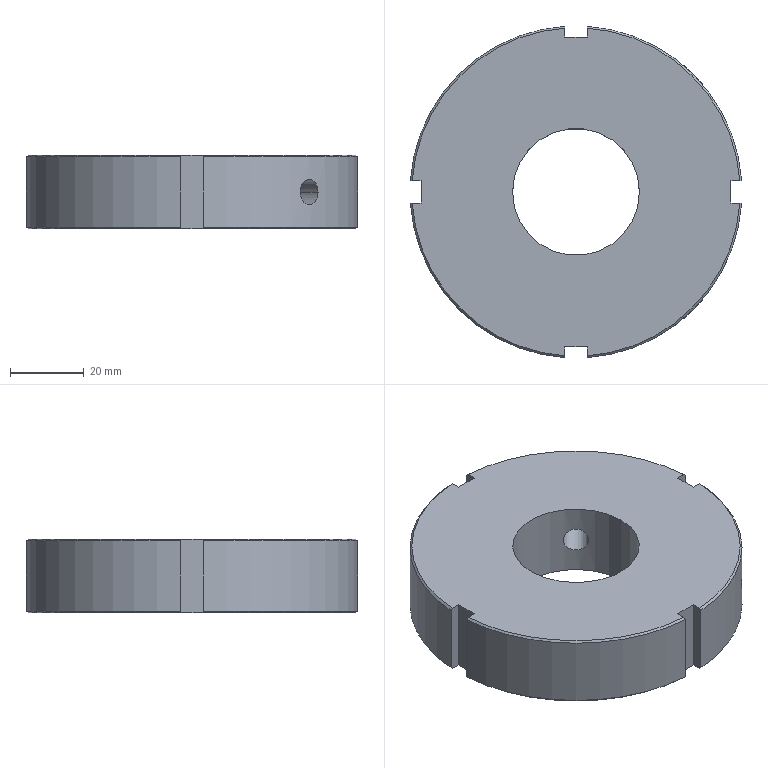Part | SolidWorks | features BaseBody 1 | 1 solid | 32 faces | box 89.8 x 89.8 x 20 mm | volume 105112 mm3 | plane 14 | cylinder 10 | cone 8 | commonest cylinder face diameters 6.88 x4 90 x4 34.376 x2
STEP:
#1=CARTESIAN_POINT('',(9.475,-14.34,0.));
#2=VERTEX_POINT('',#1);
#3=CARTESIAN_POINT('',(14.34,-9.475,0.));
#4=VERTEX_POINT('',#3);
#5=CARTESIAN_POINT('',(9.475,-14.34,0.));
#6=CARTESIAN_POINT('',(9.475,-14.34,0.2278));
#7=CARTESIAN_POINT('',(9.495,-14.328,0.4518));
#8=CARTESIAN_POINT('',(9.569,-14.278,0.8921));
#9=CARTESIAN_POINT('',(9.625,-14.241,1.111));
#10=CARTESIAN_POINT('',(9.77,-14.141,1.527));
#11=CARTESIAN_POINT('',(9.859,-14.08,1.724));
#12=CARTESIAN_POINT('',(10.065,-13.934,2.098));
#13=CARTESIAN_POINT('',(10.184,-13.847,2.274));
#14=CARTESIAN_POINT('',(10.439,-13.656,2.591));
#15=CARTESIAN_POINT('',(10.577,-13.549,2.733));
#16=CARTESIAN_POINT('',(10.873,-13.313,2.984));
#17=CARTESIAN_POINT('',(11.027,-13.186,3.091));
#18=CARTESIAN_POINT('',(11.342,-12.916,3.263));
#19=CARTESIAN_POINT('',(11.505,-12.772,3.329));
#20=CARTESIAN_POINT('',(11.832,-12.47,3.418));
#21=CARTESIAN_POINT('',(11.993,-12.315,3.44));
#22=CARTESIAN_POINT('',(12.311,-11.997,3.44));
#23=CARTESIAN_POINT('',(12.469,-11.832,3.418));
#24=CARTESIAN_POINT('',(12.769,-11.507,3.33));
#25=CARTESIAN_POINT('',(12.912,-11.347,3.265));
#26=CARTESIAN_POINT('',(13.185,-11.029,3.092));
#27=CARTESIAN_POINT('',(13.313,-10.874,2.985));
#28=CARTESIAN_POINT('',(13.546,-10.581,2.736));
#29=CARTESIAN_POINT('',(13.654,-10.442,2.593));
#30=CARTESIAN_POINT('',(13.848,-10.183,2.274));
#31=CARTESIAN_POINT('',(13.932,-10.067,2.101));
#32=CARTESIAN_POINT('',(14.079,-9.861,1.729));
#33=CARTESIAN_POINT('',(14.141,-9.771,1.528));
#34=CARTESIAN_POINT('',(14.24,-9.626,1.112));
#35=CARTESIAN_POINT('',(14.277,-9.57,0.8979));
#36=CARTESIAN_POINT('',(14.328,-9.495,0.456));
#37=CARTESIAN_POINT('',(14.34,-9.475,0.2279));
#38=CARTESIAN_POINT('',(14.34,-9.475,0.));
#39=B_SPLINE_CURVE_WITH_KNOTS('',3,(#5,#6,#7,#8,#9,#10,#11,#12,#13,#14,#15,#16,#17,#18,#19,#20,#21,#22,#23,#24,#25,#26,#27,#28,#29,#30,#31,#32,#33,#34,#35,#36,#37,#38),.UNSPECIFIED.,.F.,.F.,(4,2,2,2,2,2,2,2,2,2,2,2,2,2,2,2,4),(0.,0.0006737,0.001347,0.002021,0.002695,0.003369,0.004042,0.004716,0.00539,0.006063,0.006737,0.007411,0.008085,0.008758,0.009432,0.01011,0.01078),.UNSPECIFIED.);
#40=EDGE_CURVE('',#2,#4,#39,.T.);
#41=ORIENTED_EDGE('',*,*,#40,.F.);
#42=CARTESIAN_POINT('',(14.34,-9.475,0.));
#43=CARTESIAN_POINT('',(14.34,-9.475,-0.2278));
#44=CARTESIAN_POINT('',(14.328,-9.495,-0.4518));
#45=CARTESIAN_POINT('',(14.278,-9.569,-0.8921));
#46=CARTESIAN_POINT('',(14.241,-9.625,-1.111));
#47=CARTESIAN_POINT('',(14.141,-9.77,-1.527));
#48=CARTESIAN_POINT('',(14.08,-9.859,-1.724));
#49=CARTESIAN_POINT('',(13.934,-10.065,-2.098));
#50=CARTESIAN_POINT('',(13.847,-10.184,-2.274));
#51=CARTESIAN_POINT('',(13.656,-10.439,-2.591));
#52=CARTESIAN_POINT('',(13.549,-10.577,-2.733));
#53=CARTESIAN_POINT('',(13.313,-10.873,-2.984));
#54=CARTESIAN_POINT('',(13.186,-11.027,-3.091));
#55=CARTESIAN_POINT('',(12.916,-11.342,-3.263));
#56=CARTESIAN_POINT('',(12.772,-11.505,-3.329));
#57=CARTESIAN_POINT('',(12.47,-11.832,-3.418));
#58=CARTESIAN_POINT('',(12.315,-11.993,-3.44));
#59=CARTESIAN_POINT('',(11.997,-12.311,-3.44));
#60=CARTESIAN_POINT('',(11.832,-12.469,-3.418));
#61=CARTESIAN_POINT('',(11.507,-12.769,-3.33));
#62=CARTESIAN_POINT('',(11.347,-12.912,-3.265));
#63=CARTESIAN_POINT('',(11.029,-13.185,-3.092));
#64=CARTESIAN_POINT('',(10.874,-13.313,-2.985));
#65=CARTESIAN_POINT('',(10.581,-13.546,-2.736));
#66=CARTESIAN_POINT('',(10.442,-13.654,-2.593));
#67=CARTESIAN_POINT('',(10.183,-13.848,-2.274));
#68=CARTESIAN_POINT('',(10.067,-13.932,-2.101));
#69=CARTESIAN_POINT('',(9.861,-14.079,-1.729));
#70=CARTESIAN_POINT('',(9.771,-14.141,-1.528));
#71=CARTESIAN_POINT('',(9.626,-14.24,-1.112));
#72=CARTESIAN_POINT('',(9.57,-14.277,-0.8979));
#73=CARTESIAN_POINT('',(9.495,-14.328,-0.456));
#74=CARTESIAN_POINT('',(9.475,-14.34,-0.2278));
#75=CARTESIAN_POINT('',(9.475,-14.34,0.));
#76=B_SPLINE_CURVE_WITH_KNOTS('',3,(#42,#43,#44,#45,#46,#47,#48,#49,#50,#51,#52,#53,#54,#55,#56,#57,#58,#59,#60,#61,#62,#63,#64,#65,#66,#67,#68,#69,#70,#71,#72,#73,#74,#75),.UNSPECIFIED.,.F.,.F.,(4,2,2,2,2,2,2,2,2,2,2,2,2,2,2,2,4),(0.01078,0.01145,0.01213,0.0128,0.01347,0.01415,0.01482,0.0155,0.01617,0.01684,0.01752,0.01819,0.01886,0.01954,0.02021,0.02088,0.02156),.UNSPECIFIED.);
#77=EDGE_CURVE('',#4,#2,#76,.T.);
#78=ORIENTED_EDGE('',*,*,#77,.F.);
#79=EDGE_LOOP('',(#41,#78));
#80=FACE_BOUND('',#79,.T.);
#81=CARTESIAN_POINT('',(17.188,0.,10.));
#82=VERTEX_POINT('',#81);
#83=CARTESIAN_POINT('',(-17.188,0.,10.));
#84=VERTEX_POINT('',#83);
#85=CARTESIAN_POINT('',(0.,0.,10.));
#86=DIRECTION('',(0.,0.,-1.));
#87=DIRECTION('',(-1.,0.,0.));
#88=AXIS2_PLACEMENT_3D('',#85,#86,#87);
#89=CIRCLE('',#88,17.188);
#90=EDGE_CURVE('',#82,#84,#89,.T.);
#91=ORIENTED_EDGE('',*,*,#90,.F.);
#92=CARTESIAN_POINT('',(17.188,0.,-10.));
#93=VERTEX_POINT('',#92);
#94=CARTESIAN_POINT('',(17.188,0.,10.));
#95=DIRECTION('',(0.,0.,-1.));
#96=VECTOR('',#95,1000.);
#97=LINE('',#94,#96);
#98=EDGE_CURVE('',#82,#93,#97,.T.);
#99=ORIENTED_EDGE('',*,*,#98,.T.);
#100=CARTESIAN_POINT('',(-17.188,0.,-10.));
#101=VERTEX_POINT('',#100);
#102=CARTESIAN_POINT('',(0.,0.,-10.));
#103=DIRECTION('',(0.,0.,1.));
#104=DIRECTION('',(-1.,0.,0.));
#105=AXIS2_PLACEMENT_3D('',#102,#103,#104);
#106=CIRCLE('',#105,17.188);
#107=EDGE_CURVE('',#101,#93,#106,.T.);
#108=ORIENTED_EDGE('',*,*,#107,.F.);
#109=CARTESIAN_POINT('',(-17.188,0.,10.));
#110=DIRECTION('',(0.,0.,-1.));
#111=VECTOR('',#110,1000.);
#112=LINE('',#109,#111);
#113=EDGE_CURVE('',#84,#101,#112,.T.);
#114=ORIENTED_EDGE('',*,*,#113,.F.);
#115=EDGE_LOOP('',(#91,#99,#108,#114));
#116=FACE_OUTER_BOUND('',#115,.T.);
#117=CARTESIAN_POINT('',(0.,0.,10.));
#118=DIRECTION('',(0.,0.,-1.));
#119=DIRECTION('',(-1.,0.,0.));
#120=AXIS2_PLACEMENT_3D('',#117,#118,#119);
#121=CYLINDRICAL_SURFACE('',#120,17.188);
#122=ADVANCED_FACE('',(#80,#116),#121,.F.);
#123=CARTESIAN_POINT('',(29.294,34.159,0.));
#124=VERTEX_POINT('',#123);
#125=CARTESIAN_POINT('',(34.159,29.294,0.));
#126=VERTEX_POINT('',#125);
#127=CARTESIAN_POINT('',(29.294,34.159,0.));
#128=CARTESIAN_POINT('',(29.294,34.159,-0.2273));
#129=CARTESIAN_POINT('',(29.311,34.145,-0.4508));
#130=CARTESIAN_POINT('',(29.378,34.087,-0.8906));
#131=CARTESIAN_POINT('',(29.428,34.044,-1.109));
#132=CARTESIAN_POINT('',(29.559,33.931,-1.526));
#133=CARTESIAN_POINT('',(29.639,33.861,-1.723));
#134=CARTESIAN_POINT('',(29.826,33.696,-2.097));
#135=CARTESIAN_POINT('',(29.935,33.599,-2.274));
#136=CARTESIAN_POINT('',(30.172,33.387,-2.591));
#137=CARTESIAN_POINT('',(30.3,33.271,-2.733));
#138=CARTESIAN_POINT('',(30.577,33.016,-2.985));
#139=CARTESIAN_POINT('',(30.724,32.88,-3.092));
#140=CARTESIAN_POINT('',(31.025,32.596,-3.263));
#141=CARTESIAN_POINT('',(31.182,32.446,-3.329));
#142=CARTESIAN_POINT('',(31.5,32.137,-3.418));
#143=CARTESIAN_POINT('',(31.659,31.98,-3.44));
#144=CARTESIAN_POINT('',(31.977,31.663,-3.44));
#145=CARTESIAN_POINT('',(32.137,31.5,-3.418));
#146=CARTESIAN_POINT('',(32.444,31.184,-3.33));
#147=CARTESIAN_POINT('',(32.592,31.029,-3.265));
#148=CARTESIAN_POINT('',(32.878,30.726,-3.093));
#149=CARTESIAN_POINT('',(33.015,30.578,-2.985));
#150=CARTESIAN_POINT('',(33.268,30.303,-2.737));
#151=CARTESIAN_POINT('',(33.385,30.174,-2.595));
#152=CARTESIAN_POINT('',(33.6,29.935,-2.274));
#153=CARTESIAN_POINT('',(33.694,29.828,-2.1));
#154=CARTESIAN_POINT('',(33.859,29.641,-1.728));
#155=CARTESIAN_POINT('',(33.93,29.559,-1.527));
#156=CARTESIAN_POINT('',(34.044,29.428,-1.11));
#157=CARTESIAN_POINT('',(34.087,29.379,-0.8956));
#158=CARTESIAN_POINT('',(34.144,29.312,-0.4548));
#159=CARTESIAN_POINT('',(34.159,29.294,-0.2273));
#160=CARTESIAN_POINT('',(34.159,29.294,0.));
#161=B_SPLINE_CURVE_WITH_KNOTS('',3,(#127,#128,#129,#130,#131,#132,#133,#134,#135,#136,#137,#138,#139,#140,#141,#142,#143,#144,#145,#146,#147,#148,#149,#150,#151,#152,#153,#154,#155,#156,#157,#158,#159,#160),.UNSPECIFIED.,.F.,.F.,(4,2,2,2,2,2,2,2,2,2,2,2,2,2,2,2,4),(0.,0.0006723,0.001345,0.002017,0.002689,0.003361,0.004034,0.004706,0.005378,0.006051,0.006723,0.007395,0.008067,0.00874,0.009412,0.01008,0.01076),.UNSPECIFIED.);
#162=EDGE_CURVE('',#124,#126,#161,.T.);
#163=ORIENTED_EDGE('',*,*,#162,.F.);
#164=CARTESIAN_POINT('',(9.475,14.34,0.));
#165=VERTEX_POINT('',#164);
#166=CARTESIAN_POINT('',(42.568,47.432,0.));
#167=DIRECTION('',(-0.7071,-0.7071,0.));
#168=VECTOR('',#167,1000.);
#169=LINE('',#166,#168);
#170=EDGE_CURVE('',#124,#165,#169,.T.);
#171=ORIENTED_EDGE('',*,*,#170,.T.);
#172=CARTESIAN_POINT('',(14.34,9.475,0.));
#173=VERTEX_POINT('',#172);
#174=CARTESIAN_POINT('',(9.475,14.34,0.));
#175=CARTESIAN_POINT('',(9.475,14.34,-0.2278));
#176=CARTESIAN_POINT('',(9.495,14.328,-0.4518));
#177=CARTESIAN_POINT('',(9.569,14.278,-0.8921));
#178=CARTESIAN_POINT('',(9.625,14.241,-1.111));
#179=CARTESIAN_POINT('',(9.77,14.141,-1.527));
#180=CARTESIAN_POINT('',(9.859,14.08,-1.724));
#181=CARTESIAN_POINT('',(10.065,13.934,-2.098));
#182=CARTESIAN_POINT('',(10.184,13.847,-2.274));
#183=CARTESIAN_POINT('',(10.439,13.656,-2.591));
#184=CARTESIAN_POINT('',(10.577,13.549,-2.733));
#185=CARTESIAN_POINT('',(10.873,13.313,-2.984));
#186=CARTESIAN_POINT('',(11.027,13.186,-3.091));
#187=CARTESIAN_POINT('',(11.342,12.916,-3.263));
#188=CARTESIAN_POINT('',(11.505,12.772,-3.329));
#189=CARTESIAN_POINT('',(11.832,12.47,-3.418));
#190=CARTESIAN_POINT('',(11.993,12.315,-3.44));
#191=CARTESIAN_POINT('',(12.311,11.997,-3.44));
#192=CARTESIAN_POINT('',(12.469,11.832,-3.418));
#193=CARTESIAN_POINT('',(12.769,11.507,-3.33));
#194=CARTESIAN_POINT('',(12.912,11.347,-3.265));
#195=CARTESIAN_POINT('',(13.185,11.029,-3.092));
#196=CARTESIAN_POINT('',(13.313,10.874,-2.985));
#197=CARTESIAN_POINT('',(13.546,10.581,-2.736));
#198=CARTESIAN_POINT('',(13.654,10.442,-2.593));
#199=CARTESIAN_POINT('',(13.848,10.183,-2.274));
#200=CARTESIAN_POINT('',(13.932,10.067,-2.101));
#201=CARTESIAN_POINT('',(14.079,9.861,-1.729));
#202=CARTESIAN_POINT('',(14.141,9.771,-1.528));
#203=CARTESIAN_POINT('',(14.24,9.626,-1.112));
#204=CARTESIAN_POINT('',(14.277,9.57,-0.8979));
#205=CARTESIAN_POINT('',(14.328,9.495,-0.456));
#206=CARTESIAN_POINT('',(14.34,9.475,-0.2279));
#207=CARTESIAN_POINT('',(14.34,9.475,0.));
#208=B_SPLINE_CURVE_WITH_KNOTS('',3,(#174,#175,#176,#177,#178,#179,#180,#181,#182,#183,#184,#185,#186,#187,#188,#189,#190,#191,#192,#193,#194,#195,#196,#197,#198,#199,#200,#201,#202,#203,#204,#205,#206,#207),.UNSPECIFIED.,.F.,.F.,(4,2,2,2,2,2,2,2,2,2,2,2,2,2,2,2,4),(0.,0.0006737,0.001347,0.002021,0.002695,0.003369,0.004042,0.004716,0.00539,0.006063,0.006737,0.007411,0.008085,0.008758,0.009432,0.01011,0.01078),.UNSPECIFIED.);
#209=EDGE_CURVE('',#165,#173,#208,.T.);
#210=ORIENTED_EDGE('',*,*,#209,.T.);
#211=CARTESIAN_POINT('',(47.432,42.568,0.));
#212=DIRECTION('',(-0.7071,-0.7071,0.));
#213=VECTOR('',#212,1000.);
#214=LINE('',#211,#213);
#215=EDGE_CURVE('',#126,#173,#214,.T.);
#216=ORIENTED_EDGE('',*,*,#215,.F.);
#217=EDGE_LOOP('',(#163,#171,#210,#216));
#218=FACE_OUTER_BOUND('',#217,.T.);
#219=CARTESIAN_POINT('',(45.,45.,0.));
#220=DIRECTION('',(-0.7071,-0.7071,0.));
#221=DIRECTION('',(0.7071,-0.7071,0.));
#222=AXIS2_PLACEMENT_3D('',#219,#220,#221);
#223=CYLINDRICAL_SURFACE('',#222,3.44);
#224=ADVANCED_FACE('',(#218),#223,.F.);
#225=CARTESIAN_POINT('',(34.159,-29.294,0.));
#226=VERTEX_POINT('',#225);
#227=CARTESIAN_POINT('',(29.294,-34.159,0.));
#228=VERTEX_POINT('',#227);
#229=CARTESIAN_POINT('',(34.159,-29.294,0.));
#230=CARTESIAN_POINT('',(34.159,-29.294,-0.2273));
#231=CARTESIAN_POINT('',(34.145,-29.311,-0.4508));
#232=CARTESIAN_POINT('',(34.087,-29.378,-0.8906));
#233=CARTESIAN_POINT('',(34.044,-29.428,-1.109));
#234=CARTESIAN_POINT('',(33.931,-29.559,-1.526));
#235=CARTESIAN_POINT('',(33.861,-29.639,-1.723));
#236=CARTESIAN_POINT('',(33.696,-29.826,-2.097));
#237=CARTESIAN_POINT('',(33.599,-29.935,-2.274));
#238=CARTESIAN_POINT('',(33.387,-30.172,-2.591));
#239=CARTESIAN_POINT('',(33.271,-30.3,-2.733));
#240=CARTESIAN_POINT('',(33.016,-30.577,-2.985));
#241=CARTESIAN_POINT('',(32.88,-30.724,-3.092));
#242=CARTESIAN_POINT('',(32.596,-31.025,-3.263));
#243=CARTESIAN_POINT('',(32.446,-31.182,-3.329));
#244=CARTESIAN_POINT('',(32.137,-31.5,-3.418));
#245=CARTESIAN_POINT('',(31.98,-31.659,-3.44));
#246=CARTESIAN_POINT('',(31.663,-31.977,-3.44));
#247=CARTESIAN_POINT('',(31.5,-32.137,-3.418));
#248=CARTESIAN_POINT('',(31.184,-32.444,-3.33));
#249=CARTESIAN_POINT('',(31.029,-32.592,-3.265));
#250=CARTESIAN_POINT('',(30.726,-32.878,-3.093));
#251=CARTESIAN_POINT('',(30.578,-33.015,-2.985));
#252=CARTESIAN_POINT('',(30.303,-33.268,-2.737));
#253=CARTESIAN_POINT('',(30.174,-33.385,-2.595));
#254=CARTESIAN_POINT('',(29.935,-33.6,-2.274));
#255=CARTESIAN_POINT('',(29.828,-33.694,-2.1));
#256=CARTESIAN_POINT('',(29.641,-33.859,-1.728));
#257=CARTESIAN_POINT('',(29.559,-33.93,-1.527));
#258=CARTESIAN_POINT('',(29.428,-34.044,-1.11));
#259=CARTESIAN_POINT('',(29.379,-34.087,-0.8956));
#260=CARTESIAN_POINT('',(29.312,-34.144,-0.4548));
#261=CARTESIAN_POINT('',(29.294,-34.159,-0.2273));
#262=CARTESIAN_POINT('',(29.294,-34.159,0.));
#263=B_SPLINE_CURVE_WITH_KNOTS('',3,(#229,#230,#231,#232,#233,#234,#235,#236,#237,#238,#239,#240,#241,#242,#243,#244,#245,#246,#247,#248,#249,#250,#251,#252,#253,#254,#255,#256,#257,#258,#259,#260,#261,#262),.UNSPECIFIED.,.F.,.F.,(4,2,2,2,2,2,2,2,2,2,2,2,2,2,2,2,4),(0.01076,0.01143,0.0121,0.01277,0.01345,0.01412,0.01479,0.01546,0.01613,0.01681,0.01748,0.01815,0.01882,0.0195,0.02017,0.02084,0.02151),.UNSPECIFIED.);
#264=EDGE_CURVE('',#226,#228,#263,.T.);
#265=ORIENTED_EDGE('',*,*,#264,.F.);
#266=CARTESIAN_POINT('',(47.432,-42.568,0.));
#267=DIRECTION('',(-0.7071,0.7071,0.));
#268=VECTOR('',#267,1000.);
#269=LINE('',#266,#268);
#270=EDGE_CURVE('',#226,#4,#269,.T.);
#271=ORIENTED_EDGE('',*,*,#270,.T.);
#272=ORIENTED_EDGE('',*,*,#77,.T.);
#273=CARTESIAN_POINT('',(42.568,-47.432,0.));
#274=DIRECTION('',(-0.7071,0.7071,0.));
#275=VECTOR('',#274,1000.);
#276=LINE('',#273,#275);
#277=EDGE_CURVE('',#228,#2,#276,.T.);
#278=ORIENTED_EDGE('',*,*,#277,.F.);
#279=EDGE_LOOP('',(#265,#271,#272,#278));
#280=FACE_OUTER_BOUND('',#279,.T.);
#281=CARTESIAN_POINT('',(45.,-45.,0.));
#282=DIRECTION('',(-0.7071,0.7071,0.));
#283=DIRECTION('',(-0.7071,-0.7071,0.));
#284=AXIS2_PLACEMENT_3D('',#281,#282,#283);
#285=CYLINDRICAL_SURFACE('',#284,3.44);
#286=ADVANCED_FACE('',(#280),#285,.F.);
#287=CARTESIAN_POINT('',(0.,0.,10.));
#288=DIRECTION('',(0.,0.,-1.));
#289=DIRECTION('',(-1.,0.,0.));
#290=AXIS2_PLACEMENT_3D('',#287,#288,#289);
#291=CIRCLE('',#290,17.188);
#292=EDGE_CURVE('',#84,#82,#291,.T.);
#293=ORIENTED_EDGE('',*,*,#292,.T.);
#294=ORIENTED_EDGE('',*,*,#90,.T.);
#295=EDGE_LOOP('',(#293,#294));
#296=FACE_BOUND('',#295,.T.);
#297=CARTESIAN_POINT('',(3.,-42.,10.));
#298=VERTEX_POINT('',#297);
#299=CARTESIAN_POINT('',(3.,-44.399,10.));
#300=VERTEX_POINT('',#299);
#301=CARTESIAN_POINT('',(3.,0.,10.));
#302=DIRECTION('',(0.,-1.,0.));
#303=VECTOR('',#302,1000.);
#304=LINE('',#301,#303);
#305=EDGE_CURVE('',#298,#300,#304,.T.);
#306=ORIENTED_EDGE('',*,*,#305,.T.);
#307=CARTESIAN_POINT('',(44.399,-3.,10.));
#308=VERTEX_POINT('',#307);
#309=CARTESIAN_POINT('',(0.,0.,10.));
#310=DIRECTION('',(0.,0.,1.));
#311=DIRECTION('',(-1.,0.,0.));
#312=AXIS2_PLACEMENT_3D('',#309,#310,#311);
#313=CIRCLE('',#312,44.5);
#314=EDGE_CURVE('',#300,#308,#313,.T.);
#315=ORIENTED_EDGE('',*,*,#314,.T.);
#316=CARTESIAN_POINT('',(42.,-3.,10.));
#317=VERTEX_POINT('',#316);
#318=CARTESIAN_POINT('',(0.,-3.,10.));
#319=DIRECTION('',(-1.,0.,0.));
#320=VECTOR('',#319,1000.);
#321=LINE('',#318,#320);
#322=EDGE_CURVE('',#308,#317,#321,.T.);
#323=ORIENTED_EDGE('',*,*,#322,.T.);
#324=CARTESIAN_POINT('',(42.,3.,10.));
#325=VERTEX_POINT('',#324);
#326=CARTESIAN_POINT('',(42.,0.,10.));
#327=DIRECTION('',(0.,1.,0.));
#328=VECTOR('',#327,1000.);
#329=LINE('',#326,#328);
#330=EDGE_CURVE('',#317,#325,#329,.T.);
#331=ORIENTED_EDGE('',*,*,#330,.T.);
#332=CARTESIAN_POINT('',(44.399,3.,10.));
#333=VERTEX_POINT('',#332);
#334=CARTESIAN_POINT('',(0.,3.,10.));
#335=DIRECTION('',(1.,0.,0.));
#336=VECTOR('',#335,1000.);
#337=LINE('',#334,#336);
#338=EDGE_CURVE('',#325,#333,#337,.T.);
#339=ORIENTED_EDGE('',*,*,#338,.T.);
#340=CARTESIAN_POINT('',(3.,44.399,10.));
#341=VERTEX_POINT('',#340);
#342=CARTESIAN_POINT('',(0.,0.,10.));
#343=DIRECTION('',(0.,0.,1.));
#344=DIRECTION('',(0.,1.,0.));
#345=AXIS2_PLACEMENT_3D('',#342,#343,#344);
#346=CIRCLE('',#345,44.5);
#347=EDGE_CURVE('',#333,#341,#346,.T.);
#348=ORIENTED_EDGE('',*,*,#347,.T.);
#349=CARTESIAN_POINT('',(3.,42.,10.));
#350=VERTEX_POINT('',#349);
#351=CARTESIAN_POINT('',(3.,0.,10.));
#352=DIRECTION('',(0.,-1.,0.));
#353=VECTOR('',#352,1000.);
#354=LINE('',#351,#353);
#355=EDGE_CURVE('',#341,#350,#354,.T.);
#356=ORIENTED_EDGE('',*,*,#355,.T.);
#357=CARTESIAN_POINT('',(-3.,42.,10.));
#358=VERTEX_POINT('',#357);
#359=CARTESIAN_POINT('',(0.,42.,10.));
#360=DIRECTION('',(-1.,0.,0.));
#361=VECTOR('',#360,1000.);
#362=LINE('',#359,#361);
#363=EDGE_CURVE('',#350,#358,#362,.T.);
#364=ORIENTED_EDGE('',*,*,#363,.T.);
#365=CARTESIAN_POINT('',(-3.,44.399,10.));
#366=VERTEX_POINT('',#365);
#367=CARTESIAN_POINT('',(-3.,0.,10.));
#368=DIRECTION('',(0.,1.,0.));
#369=VECTOR('',#368,1000.);
#370=LINE('',#367,#369);
#371=EDGE_CURVE('',#358,#366,#370,.T.);
#372=ORIENTED_EDGE('',*,*,#371,.T.);
#373=CARTESIAN_POINT('',(-44.399,3.,10.));
#374=VERTEX_POINT('',#373);
#375=CARTESIAN_POINT('',(0.,0.,10.));
#376=DIRECTION('',(0.,0.,1.));
#377=DIRECTION('',(-1.,0.,0.));
#378=AXIS2_PLACEMENT_3D('',#375,#376,#377);
#379=CIRCLE('',#378,44.5);
#380=EDGE_CURVE('',#366,#374,#379,.T.);
#381=ORIENTED_EDGE('',*,*,#380,.T.);
#382=CARTESIAN_POINT('',(-42.,3.,10.));
#383=VERTEX_POINT('',#382);
#384=CARTESIAN_POINT('',(0.,3.,10.));
#385=DIRECTION('',(1.,0.,0.));
#386=VECTOR('',#385,1000.);
#387=LINE('',#384,#386);
#388=EDGE_CURVE('',#374,#383,#387,.T.);
#389=ORIENTED_EDGE('',*,*,#388,.T.);
#390=CARTESIAN_POINT('',(-42.,-3.,10.));
#391=VERTEX_POINT('',#390);
#392=CARTESIAN_POINT('',(-42.,0.,10.));
#393=DIRECTION('',(0.,-1.,0.));
#394=VECTOR('',#393,1000.);
#395=LINE('',#392,#394);
#396=EDGE_CURVE('',#383,#391,#395,.T.);
#397=ORIENTED_EDGE('',*,*,#396,.T.);
#398=CARTESIAN_POINT('',(-44.399,-3.,10.));
#399=VERTEX_POINT('',#398);
#400=CARTESIAN_POINT('',(0.,-3.,10.));
#401=DIRECTION('',(-1.,0.,0.));
#402=VECTOR('',#401,1000.);
#403=LINE('',#400,#402);
#404=EDGE_CURVE('',#391,#399,#403,.T.);
#405=ORIENTED_EDGE('',*,*,#404,.T.);
#406=CARTESIAN_POINT('',(-3.,-44.399,10.));
#407=VERTEX_POINT('',#406);
#408=CARTESIAN_POINT('',(0.,0.,10.));
#409=DIRECTION('',(0.,0.,1.));
#410=DIRECTION('',(-1.,0.,0.));
#411=AXIS2_PLACEMENT_3D('',#408,#409,#410);
#412=CIRCLE('',#411,44.5);
#413=EDGE_CURVE('',#399,#407,#412,.T.);
#414=ORIENTED_EDGE('',*,*,#413,.T.);
#415=CARTESIAN_POINT('',(-3.,-42.,10.));
#416=VERTEX_POINT('',#415);
#417=CARTESIAN_POINT('',(-3.,0.,10.));
#418=DIRECTION('',(0.,1.,0.));
#419=VECTOR('',#418,1000.);
#420=LINE('',#417,#419);
#421=EDGE_CURVE('',#407,#416,#420,.T.);
#422=ORIENTED_EDGE('',*,*,#421,.T.);
#423=CARTESIAN_POINT('',(0.,-42.,10.));
#424=DIRECTION('',(1.,0.,0.));
#425=VECTOR('',#424,1000.);
#426=LINE('',#423,#425);
#427=EDGE_CURVE('',#416,#298,#426,.T.);
#428=ORIENTED_EDGE('',*,*,#427,.T.);
#429=EDGE_LOOP('',(#306,#315,#323,#331,#339,#348,#356,#364,#372,#381,#389,#397,#405,#414,#422,#428));
#430=FACE_OUTER_BOUND('',#429,.T.);
#431=CARTESIAN_POINT('',(0.,0.,10.));
#432=DIRECTION('',(0.,0.,1.));
#433=DIRECTION('',(1.,0.,0.));
#434=AXIS2_PLACEMENT_3D('',#431,#432,#433);
#435=PLANE('',#434);
#436=ADVANCED_FACE('',(#296,#430),#435,.T.);
#437=ORIENTED_EDGE('',*,*,#98,.F.);
#438=ORIENTED_EDGE('',*,*,#292,.F.);
#439=ORIENTED_EDGE('',*,*,#113,.T.);
#440=CARTESIAN_POINT('',(0.,0.,-10.));
#441=DIRECTION('',(0.,0.,1.));
#442=DIRECTION('',(-1.,0.,0.));
#443=AXIS2_PLACEMENT_3D('',#440,#441,#442);
#444=CIRCLE('',#443,17.188);
#445=EDGE_CURVE('',#93,#101,#444,.T.);
#446=ORIENTED_EDGE('',*,*,#445,.F.);
#447=EDGE_LOOP('',(#437,#438,#439,#446));
#448=FACE_OUTER_BOUND('',#447,.T.);
#449=CARTESIAN_POINT('',(14.34,9.475,0.));
#450=CARTESIAN_POINT('',(14.34,9.475,0.2278));
#451=CARTESIAN_POINT('',(14.328,9.495,0.4518));
#452=CARTESIAN_POINT('',(14.278,9.569,0.8921));
#453=CARTESIAN_POINT('',(14.241,9.625,1.111));
#454=CARTESIAN_POINT('',(14.141,9.77,1.527));
#455=CARTESIAN_POINT('',(14.08,9.859,1.724));
#456=CARTESIAN_POINT('',(13.934,10.065,2.098));
#457=CARTESIAN_POINT('',(13.847,10.184,2.274));
#458=CARTESIAN_POINT('',(13.656,10.439,2.591));
#459=CARTESIAN_POINT('',(13.549,10.577,2.733));
#460=CARTESIAN_POINT('',(13.313,10.873,2.984));
#461=CARTESIAN_POINT('',(13.186,11.027,3.091));
#462=CARTESIAN_POINT('',(12.916,11.342,3.263));
#463=CARTESIAN_POINT('',(12.772,11.505,3.329));
#464=CARTESIAN_POINT('',(12.47,11.832,3.418));
#465=CARTESIAN_POINT('',(12.315,11.993,3.44));
#466=CARTESIAN_POINT('',(11.997,12.311,3.44));
#467=CARTESIAN_POINT('',(11.832,12.469,3.418));
#468=CARTESIAN_POINT('',(11.507,12.769,3.33));
#469=CARTESIAN_POINT('',(11.347,12.912,3.265));
#470=CARTESIAN_POINT('',(11.029,13.185,3.092));
#471=CARTESIAN_POINT('',(10.874,13.313,2.985));
#472=CARTESIAN_POINT('',(10.581,13.546,2.736));
#473=CARTESIAN_POINT('',(10.442,13.654,2.593));
#474=CARTESIAN_POINT('',(10.183,13.848,2.274));
#475=CARTESIAN_POINT('',(10.067,13.932,2.101));
#476=CARTESIAN_POINT('',(9.861,14.079,1.729));
#477=CARTESIAN_POINT('',(9.771,14.141,1.528));
#478=CARTESIAN_POINT('',(9.626,14.24,1.112));
#479=CARTESIAN_POINT('',(9.57,14.277,0.8979));
#480=CARTESIAN_POINT('',(9.495,14.328,0.456));
#481=CARTESIAN_POINT('',(9.475,14.34,0.2278));
#482=CARTESIAN_POINT('',(9.475,14.34,0.));
#483=B_SPLINE_CURVE_WITH_KNOTS('',3,(#449,#450,#451,#452,#453,#454,#455,#456,#457,#458,#459,#460,#461,#462,#463,#464,#465,#466,#467,#468,#469,#470,#471,#472,#473,#474,#475,#476,#477,#478,#479,#480,#481,#482),.UNSPECIFIED.,.F.,.F.,(4,2,2,2,2,2,2,2,2,2,2,2,2,2,2,2,4),(0.01078,0.01145,0.01213,0.0128,0.01347,0.01415,0.01482,0.0155,0.01617,0.01684,0.01752,0.01819,0.01886,0.01954,0.02021,0.02088,0.02156),.UNSPECIFIED.);
#484=EDGE_CURVE('',#173,#165,#483,.T.);
#485=ORIENTED_EDGE('',*,*,#484,.F.);
#486=ORIENTED_EDGE('',*,*,#209,.F.);
#487=EDGE_LOOP('',(#485,#486));
#488=FACE_BOUND('',#487,.T.);
#489=CARTESIAN_POINT('',(0.,0.,10.));
#490=DIRECTION('',(0.,0.,-1.));
#491=DIRECTION('',(-1.,0.,0.));
#492=AXIS2_PLACEMENT_3D('',#489,#490,#491);
#493=CYLINDRICAL_SURFACE('',#492,17.188);
#494=ADVANCED_FACE('',(#448,#488),#493,.F.);
#495=CARTESIAN_POINT('',(3.,-44.9,9.5));
#496=VERTEX_POINT('',#495);
#497=CARTESIAN_POINT('',(3.,-44.399,10.));
#498=CARTESIAN_POINT('',(3.,-44.566,9.833));
#499=CARTESIAN_POINT('',(3.,-44.733,9.667));
#500=CARTESIAN_POINT('',(3.,-44.9,9.5));
#501=B_SPLINE_CURVE_WITH_KNOTS('',3,(#497,#498,#499,#500),.UNSPECIFIED.,.F.,.F.,(4,4),(0.,0.0007079),.UNSPECIFIED.);
#502=EDGE_CURVE('',#300,#496,#501,.T.);
#503=ORIENTED_EDGE('',*,*,#502,.T.);
#504=CARTESIAN_POINT('',(44.9,-3.,9.5));
#505=VERTEX_POINT('',#504);
#506=CARTESIAN_POINT('',(0.,0.,9.5));
#507=DIRECTION('',(0.,0.,1.));
#508=DIRECTION('',(-1.,0.,0.));
#509=AXIS2_PLACEMENT_3D('',#506,#507,#508);
#510=CIRCLE('',#509,45.);
#511=EDGE_CURVE('',#496,#505,#510,.T.);
#512=ORIENTED_EDGE('',*,*,#511,.T.);
#513=CARTESIAN_POINT('',(44.9,-3.,9.5));
#514=CARTESIAN_POINT('',(44.733,-3.,9.667));
#515=CARTESIAN_POINT('',(44.566,-3.,9.833));
#516=CARTESIAN_POINT('',(44.399,-3.,10.));
#517=B_SPLINE_CURVE_WITH_KNOTS('',3,(#513,#514,#515,#516),.UNSPECIFIED.,.F.,.F.,(4,4),(0.,0.0007079),.UNSPECIFIED.);
#518=EDGE_CURVE('',#505,#308,#517,.T.);
#519=ORIENTED_EDGE('',*,*,#518,.T.);
#520=ORIENTED_EDGE('',*,*,#314,.F.);
#521=EDGE_LOOP('',(#503,#512,#519,#520));
#522=FACE_OUTER_BOUND('',#521,.T.);
#523=CARTESIAN_POINT('',(0.,0.,9.5));
#524=DIRECTION('',(0.,0.,-1.));
#525=DIRECTION('',(-1.,0.,0.));
#526=AXIS2_PLACEMENT_3D('',#523,#524,#525);
#527=CONICAL_SURFACE('',#526,45.,0.7854);
#528=ADVANCED_FACE('',(#522),#527,.T.);
#529=CARTESIAN_POINT('',(3.,-44.9,-9.5));
#530=VERTEX_POINT('',#529);
#531=CARTESIAN_POINT('',(3.,-44.9,-12.));
#532=DIRECTION('',(0.,0.,-1.));
#533=VECTOR('',#532,1000.);
#534=LINE('',#531,#533);
#535=EDGE_CURVE('',#496,#530,#534,.T.);
#536=ORIENTED_EDGE('',*,*,#535,.F.);
#537=ORIENTED_EDGE('',*,*,#502,.F.);
#538=ORIENTED_EDGE('',*,*,#305,.F.);
#539=CARTESIAN_POINT('',(3.,-42.,-10.));
#540=VERTEX_POINT('',#539);
#541=CARTESIAN_POINT('',(3.,-42.,-12.));
#542=DIRECTION('',(0.,0.,1.));
#543=VECTOR('',#542,1000.);
#544=LINE('',#541,#543);
#545=EDGE_CURVE('',#540,#298,#544,.T.);
#546=ORIENTED_EDGE('',*,*,#545,.F.);
#547=CARTESIAN_POINT('',(3.,-44.399,-10.));
#548=VERTEX_POINT('',#547);
#549=CARTESIAN_POINT('',(3.,-48.,-10.));
#550=DIRECTION('',(0.,1.,0.));
#551=VECTOR('',#550,1000.);
#552=LINE('',#549,#551);
#553=EDGE_CURVE('',#548,#540,#552,.T.);
#554=ORIENTED_EDGE('',*,*,#553,.F.);
#555=CARTESIAN_POINT('',(3.,-44.9,-9.5));
#556=CARTESIAN_POINT('',(3.,-44.733,-9.667));
#557=CARTESIAN_POINT('',(3.,-44.566,-9.833));
#558=CARTESIAN_POINT('',(3.,-44.399,-10.));
#559=B_SPLINE_CURVE_WITH_KNOTS('',3,(#555,#556,#557,#558),.UNSPECIFIED.,.F.,.F.,(4,4),(0.,0.0007079),.UNSPECIFIED.);
#560=EDGE_CURVE('',#530,#548,#559,.T.);
#561=ORIENTED_EDGE('',*,*,#560,.F.);
#562=EDGE_LOOP('',(#536,#537,#538,#546,#554,#561));
#563=FACE_OUTER_BOUND('',#562,.T.);
#564=CARTESIAN_POINT('',(3.,-48.,-12.));
#565=DIRECTION('',(1.,0.,0.));
#566=DIRECTION('',(0.,1.,0.));
#567=AXIS2_PLACEMENT_3D('',#564,#565,#566);
#568=PLANE('',#567);
#569=ADVANCED_FACE('',(#563),#568,.F.);
#570=ORIENTED_EDGE('',*,*,#427,.F.);
#571=CARTESIAN_POINT('',(-3.,-42.,-10.));
#572=VERTEX_POINT('',#571);
#573=CARTESIAN_POINT('',(-3.,-42.,-12.));
#574=DIRECTION('',(0.,0.,1.));
#575=VECTOR('',#574,1000.);
#576=LINE('',#573,#575);
#577=EDGE_CURVE('',#572,#416,#576,.T.);
#578=ORIENTED_EDGE('',*,*,#577,.F.);
#579=CARTESIAN_POINT('',(3.,-42.,-10.));
#580=DIRECTION('',(-1.,0.,0.));
#581=VECTOR('',#580,1000.);
#582=LINE('',#579,#581);
#583=EDGE_CURVE('',#540,#572,#582,.T.);
#584=ORIENTED_EDGE('',*,*,#583,.F.);
#585=ORIENTED_EDGE('',*,*,#545,.T.);
#586=EDGE_LOOP('',(#570,#578,#584,#585));
#587=FACE_OUTER_BOUND('',#586,.T.);
#588=CARTESIAN_POINT('',(3.,-42.,-12.));
#589=DIRECTION('',(0.,1.,0.));
#590=DIRECTION('',(0.,0.,1.));
#591=AXIS2_PLACEMENT_3D('',#588,#589,#590);
#592=PLANE('',#591);
#593=ADVANCED_FACE('',(#587),#592,.F.);
#594=ORIENTED_EDGE('',*,*,#421,.F.);
#595=CARTESIAN_POINT('',(-3.,-44.9,9.5));
#596=VERTEX_POINT('',#595);
#597=CARTESIAN_POINT('',(-3.,-44.9,9.5));
#598=CARTESIAN_POINT('',(-3.,-44.733,9.667));
#599=CARTESIAN_POINT('',(-3.,-44.566,9.833));
#600=CARTESIAN_POINT('',(-3.,-44.399,10.));
#601=B_SPLINE_CURVE_WITH_KNOTS('',3,(#597,#598,#599,#600),.UNSPECIFIED.,.F.,.F.,(4,4),(0.,0.0007079),.UNSPECIFIED.);
#602=EDGE_CURVE('',#596,#407,#601,.T.);
#603=ORIENTED_EDGE('',*,*,#602,.F.);
#604=CARTESIAN_POINT('',(-3.,-44.9,-9.5));
#605=VERTEX_POINT('',#604);
#606=CARTESIAN_POINT('',(-3.,-44.9,-12.));
#607=DIRECTION('',(0.,0.,1.));
#608=VECTOR('',#607,1000.);
#609=LINE('',#606,#608);
#610=EDGE_CURVE('',#605,#596,#609,.T.);
#611=ORIENTED_EDGE('',*,*,#610,.F.);
#612=CARTESIAN_POINT('',(-3.,-44.399,-10.));
#613=VERTEX_POINT('',#612);
#614=CARTESIAN_POINT('',(-3.,-44.399,-10.));
#615=CARTESIAN_POINT('',(-3.,-44.566,-9.833));
#616=CARTESIAN_POINT('',(-3.,-44.733,-9.667));
#617=CARTESIAN_POINT('',(-3.,-44.9,-9.5));
#618=B_SPLINE_CURVE_WITH_KNOTS('',3,(#614,#615,#616,#617),.UNSPECIFIED.,.F.,.F.,(4,4),(0.,0.0007079),.UNSPECIFIED.);
#619=EDGE_CURVE('',#613,#605,#618,.T.);
#620=ORIENTED_EDGE('',*,*,#619,.F.);
#621=CARTESIAN_POINT('',(-3.,-48.,-10.));
#622=DIRECTION('',(0.,-1.,0.));
#623=VECTOR('',#622,1000.);
#624=LINE('',#621,#623);
#625=EDGE_CURVE('',#572,#613,#624,.T.);
#626=ORIENTED_EDGE('',*,*,#625,.F.);
#627=ORIENTED_EDGE('',*,*,#577,.T.);
#628=EDGE_LOOP('',(#594,#603,#611,#620,#626,#627));
#629=FACE_OUTER_BOUND('',#628,.T.);
#630=CARTESIAN_POINT('',(-3.,-48.,-12.));
#631=DIRECTION('',(-1.,0.,0.));
#632=DIRECTION('',(0.,0.,1.));
#633=AXIS2_PLACEMENT_3D('',#630,#631,#632);
#634=PLANE('',#633);
#635=ADVANCED_FACE('',(#629),#634,.F.);
#636=CARTESIAN_POINT('',(-44.9,-3.,9.5));
#637=VERTEX_POINT('',#636);
#638=CARTESIAN_POINT('',(-44.399,-3.,10.));
#639=CARTESIAN_POINT('',(-44.566,-3.,9.833));
#640=CARTESIAN_POINT('',(-44.733,-3.,9.667));
#641=CARTESIAN_POINT('',(-44.9,-3.,9.5));
#642=B_SPLINE_CURVE_WITH_KNOTS('',3,(#638,#639,#640,#641),.UNSPECIFIED.,.F.,.F.,(4,4),(0.,0.0007079),.UNSPECIFIED.);
#643=EDGE_CURVE('',#399,#637,#642,.T.);
#644=ORIENTED_EDGE('',*,*,#643,.T.);
#645=CARTESIAN_POINT('',(0.,0.,9.5));
#646=DIRECTION('',(0.,0.,1.));
#647=DIRECTION('',(-1.,0.,0.));
#648=AXIS2_PLACEMENT_3D('',#645,#646,#647);
#649=CIRCLE('',#648,45.);
#650=EDGE_CURVE('',#637,#596,#649,.T.);
#651=ORIENTED_EDGE('',*,*,#650,.T.);
#652=ORIENTED_EDGE('',*,*,#602,.T.);
#653=ORIENTED_EDGE('',*,*,#413,.F.);
#654=EDGE_LOOP('',(#644,#651,#652,#653));
#655=FACE_OUTER_BOUND('',#654,.T.);
#656=CARTESIAN_POINT('',(0.,0.,9.5));
#657=DIRECTION('',(0.,0.,-1.));
#658=DIRECTION('',(-1.,0.,0.));
#659=AXIS2_PLACEMENT_3D('',#656,#657,#658);
#660=CONICAL_SURFACE('',#659,45.,0.7854);
#661=ADVANCED_FACE('',(#655),#660,.T.);
#662=CARTESIAN_POINT('',(-44.9,-3.,-9.5));
#663=VERTEX_POINT('',#662);
#664=CARTESIAN_POINT('',(-44.9,-3.,-12.));
#665=DIRECTION('',(0.,0.,-1.));
#666=VECTOR('',#665,1000.);
#667=LINE('',#664,#666);
#668=EDGE_CURVE('',#637,#663,#667,.T.);
#669=ORIENTED_EDGE('',*,*,#668,.F.);
#670=ORIENTED_EDGE('',*,*,#643,.F.);
#671=ORIENTED_EDGE('',*,*,#404,.F.);
#672=CARTESIAN_POINT('',(-42.,-3.,-10.));
#673=VERTEX_POINT('',#672);
#674=CARTESIAN_POINT('',(-42.,-3.,-12.));
#675=DIRECTION('',(0.,0.,1.));
#676=VECTOR('',#675,1000.);
#677=LINE('',#674,#676);
#678=EDGE_CURVE('',#673,#391,#677,.T.);
#679=ORIENTED_EDGE('',*,*,#678,.F.);
#680=CARTESIAN_POINT('',(-44.399,-3.,-10.));
#681=VERTEX_POINT('',#680);
#682=CARTESIAN_POINT('',(-48.,-3.,-10.));
#683=DIRECTION('',(1.,0.,0.));
#684=VECTOR('',#683,1000.);
#685=LINE('',#682,#684);
#686=EDGE_CURVE('',#681,#673,#685,.T.);
#687=ORIENTED_EDGE('',*,*,#686,.F.);
#688=CARTESIAN_POINT('',(-44.9,-3.,-9.5));
#689=CARTESIAN_POINT('',(-44.733,-3.,-9.667));
#690=CARTESIAN_POINT('',(-44.566,-3.,-9.833));
#691=CARTESIAN_POINT('',(-44.399,-3.,-10.));
#692=B_SPLINE_CURVE_WITH_KNOTS('',3,(#688,#689,#690,#691),.UNSPECIFIED.,.F.,.F.,(4,4),(0.,0.0007079),.UNSPECIFIED.);
#693=EDGE_CURVE('',#663,#681,#692,.T.);
#694=ORIENTED_EDGE('',*,*,#693,.F.);
#695=EDGE_LOOP('',(#669,#670,#671,#679,#687,#694));
#696=FACE_OUTER_BOUND('',#695,.T.);
#697=CARTESIAN_POINT('',(-48.,-3.,-12.));
#698=DIRECTION('',(0.,-1.,0.));
#699=DIRECTION('',(1.,0.,0.));
#700=AXIS2_PLACEMENT_3D('',#697,#698,#699);
#701=PLANE('',#700);
#702=ADVANCED_FACE('',(#696),#701,.F.);
#703=ORIENTED_EDGE('',*,*,#396,.F.);
#704=CARTESIAN_POINT('',(-42.,3.,-10.));
#705=VERTEX_POINT('',#704);
#706=CARTESIAN_POINT('',(-42.,3.,-12.));
#707=DIRECTION('',(0.,0.,1.));
#708=VECTOR('',#707,1000.);
#709=LINE('',#706,#708);
#710=EDGE_CURVE('',#705,#383,#709,.T.);
#711=ORIENTED_EDGE('',*,*,#710,.F.);
#712=CARTESIAN_POINT('',(-42.,-3.,-10.));
#713=DIRECTION('',(0.,1.,0.));
#714=VECTOR('',#713,1000.);
#715=LINE('',#712,#714);
#716=EDGE_CURVE('',#673,#705,#715,.T.);
#717=ORIENTED_EDGE('',*,*,#716,.F.);
#718=ORIENTED_EDGE('',*,*,#678,.T.);
#719=EDGE_LOOP('',(#703,#711,#717,#718));
#720=FACE_OUTER_BOUND('',#719,.T.);
#721=CARTESIAN_POINT('',(-42.,-3.,-12.));
#722=DIRECTION('',(1.,0.,0.));
#723=DIRECTION('',(0.,1.,0.));
#724=AXIS2_PLACEMENT_3D('',#721,#722,#723);
#725=PLANE('',#724);
#726=ADVANCED_FACE('',(#720),#725,.F.);
#727=ORIENTED_EDGE('',*,*,#388,.F.);
#728=CARTESIAN_POINT('',(-44.9,3.,9.5));
#729=VERTEX_POINT('',#728);
#730=CARTESIAN_POINT('',(-44.9,3.,9.5));
#731=CARTESIAN_POINT('',(-44.733,3.,9.667));
#732=CARTESIAN_POINT('',(-44.566,3.,9.833));
#733=CARTESIAN_POINT('',(-44.399,3.,10.));
#734=B_SPLINE_CURVE_WITH_KNOTS('',3,(#730,#731,#732,#733),.UNSPECIFIED.,.F.,.F.,(4,4),(0.,0.0007079),.UNSPECIFIED.);
#735=EDGE_CURVE('',#729,#374,#734,.T.);
#736=ORIENTED_EDGE('',*,*,#735,.F.);
#737=CARTESIAN_POINT('',(-44.9,3.,-9.5));
#738=VERTEX_POINT('',#737);
#739=CARTESIAN_POINT('',(-44.9,3.,-12.));
#740=DIRECTION('',(0.,0.,1.));
#741=VECTOR('',#740,1000.);
#742=LINE('',#739,#741);
#743=EDGE_CURVE('',#738,#729,#742,.T.);
#744=ORIENTED_EDGE('',*,*,#743,.F.);
#745=CARTESIAN_POINT('',(-44.399,3.,-10.));
#746=VERTEX_POINT('',#745);
#747=CARTESIAN_POINT('',(-44.399,3.,-10.));
#748=CARTESIAN_POINT('',(-44.566,3.,-9.833));
#749=CARTESIAN_POINT('',(-44.733,3.,-9.667));
#750=CARTESIAN_POINT('',(-44.9,3.,-9.5));
#751=B_SPLINE_CURVE_WITH_KNOTS('',3,(#747,#748,#749,#750),.UNSPECIFIED.,.F.,.F.,(4,4),(0.,0.0007079),.UNSPECIFIED.);
#752=EDGE_CURVE('',#746,#738,#751,.T.);
#753=ORIENTED_EDGE('',*,*,#752,.F.);
#754=CARTESIAN_POINT('',(-48.,3.,-10.));
#755=DIRECTION('',(-1.,0.,0.));
#756=VECTOR('',#755,1000.);
#757=LINE('',#754,#756);
#758=EDGE_CURVE('',#705,#746,#757,.T.);
#759=ORIENTED_EDGE('',*,*,#758,.F.);
#760=ORIENTED_EDGE('',*,*,#710,.T.);
#761=EDGE_LOOP('',(#727,#736,#744,#753,#759,#760));
#762=FACE_OUTER_BOUND('',#761,.T.);
#763=CARTESIAN_POINT('',(-48.,3.,-12.));
#764=DIRECTION('',(0.,1.,0.));
#765=DIRECTION('',(-1.,0.,0.));
#766=AXIS2_PLACEMENT_3D('',#763,#764,#765);
#767=PLANE('',#766);
#768=ADVANCED_FACE('',(#762),#767,.F.);
#769=CARTESIAN_POINT('',(-3.,44.9,9.5));
#770=VERTEX_POINT('',#769);
#771=CARTESIAN_POINT('',(-3.,44.399,10.));
#772=CARTESIAN_POINT('',(-3.,44.566,9.833));
#773=CARTESIAN_POINT('',(-3.,44.733,9.667));
#774=CARTESIAN_POINT('',(-3.,44.9,9.5));
#775=B_SPLINE_CURVE_WITH_KNOTS('',3,(#771,#772,#773,#774),.UNSPECIFIED.,.F.,.F.,(4,4),(0.,0.0007079),.UNSPECIFIED.);
#776=EDGE_CURVE('',#366,#770,#775,.T.);
#777=ORIENTED_EDGE('',*,*,#776,.T.);
#778=CARTESIAN_POINT('',(0.,0.,9.5));
#779=DIRECTION('',(0.,0.,1.));
#780=DIRECTION('',(-1.,0.,0.));
#781=AXIS2_PLACEMENT_3D('',#778,#779,#780);
#782=CIRCLE('',#781,45.);
#783=EDGE_CURVE('',#770,#729,#782,.T.);
#784=ORIENTED_EDGE('',*,*,#783,.T.);
#785=ORIENTED_EDGE('',*,*,#735,.T.);
#786=ORIENTED_EDGE('',*,*,#380,.F.);
#787=EDGE_LOOP('',(#777,#784,#785,#786));
#788=FACE_OUTER_BOUND('',#787,.T.);
#789=CARTESIAN_POINT('',(0.,0.,9.5));
#790=DIRECTION('',(0.,0.,-1.));
#791=DIRECTION('',(-1.,0.,0.));
#792=AXIS2_PLACEMENT_3D('',#789,#790,#791);
#793=CONICAL_SURFACE('',#792,45.,0.7854);
#794=ADVANCED_FACE('',(#788),#793,.T.);
#795=CARTESIAN_POINT('',(-3.,44.9,-9.5));
#796=VERTEX_POINT('',#795);
#797=CARTESIAN_POINT('',(-3.,44.9,-12.));
#798=DIRECTION('',(0.,0.,-1.));
#799=VECTOR('',#798,1000.);
#800=LINE('',#797,#799);
#801=EDGE_CURVE('',#770,#796,#800,.T.);
#802=ORIENTED_EDGE('',*,*,#801,.F.);
#803=ORIENTED_EDGE('',*,*,#776,.F.);
#804=ORIENTED_EDGE('',*,*,#371,.F.);
#805=CARTESIAN_POINT('',(-3.,42.,-10.));
#806=VERTEX_POINT('',#805);
#807=CARTESIAN_POINT('',(-3.,42.,-12.));
#808=DIRECTION('',(0.,0.,1.));
#809=VECTOR('',#808,1000.);
#810=LINE('',#807,#809);
#811=EDGE_CURVE('',#806,#358,#810,.T.);
#812=ORIENTED_EDGE('',*,*,#811,.F.);
#813=CARTESIAN_POINT('',(-3.,44.399,-10.));
#814=VERTEX_POINT('',#813);
#815=CARTESIAN_POINT('',(-3.,48.,-10.));
#816=DIRECTION('',(0.,-1.,0.));
#817=VECTOR('',#816,1000.);
#818=LINE('',#815,#817);
#819=EDGE_CURVE('',#814,#806,#818,.T.);
#820=ORIENTED_EDGE('',*,*,#819,.F.);
#821=CARTESIAN_POINT('',(-3.,44.9,-9.5));
#822=CARTESIAN_POINT('',(-3.,44.733,-9.667));
#823=CARTESIAN_POINT('',(-3.,44.566,-9.833));
#824=CARTESIAN_POINT('',(-3.,44.399,-10.));
#825=B_SPLINE_CURVE_WITH_KNOTS('',3,(#821,#822,#823,#824),.UNSPECIFIED.,.F.,.F.,(4,4),(0.,0.0007079),.UNSPECIFIED.);
#826=EDGE_CURVE('',#796,#814,#825,.T.);
#827=ORIENTED_EDGE('',*,*,#826,.F.);
#828=EDGE_LOOP('',(#802,#803,#804,#812,#820,#827));
#829=FACE_OUTER_BOUND('',#828,.T.);
#830=CARTESIAN_POINT('',(-3.,48.,-12.));
#831=DIRECTION('',(-1.,0.,0.));
#832=DIRECTION('',(0.,-1.,0.));
#833=AXIS2_PLACEMENT_3D('',#830,#831,#832);
#834=PLANE('',#833);
#835=ADVANCED_FACE('',(#829),#834,.F.);
#836=ORIENTED_EDGE('',*,*,#363,.F.);
#837=CARTESIAN_POINT('',(3.,42.,-10.));
#838=VERTEX_POINT('',#837);
#839=CARTESIAN_POINT('',(3.,42.,-12.));
#840=DIRECTION('',(0.,0.,1.));
#841=VECTOR('',#840,1000.);
#842=LINE('',#839,#841);
#843=EDGE_CURVE('',#838,#350,#842,.T.);
#844=ORIENTED_EDGE('',*,*,#843,.F.);
#845=CARTESIAN_POINT('',(-3.,42.,-10.));
#846=DIRECTION('',(1.,0.,0.));
#847=VECTOR('',#846,1000.);
#848=LINE('',#845,#847);
#849=EDGE_CURVE('',#806,#838,#848,.T.);
#850=ORIENTED_EDGE('',*,*,#849,.F.);
#851=ORIENTED_EDGE('',*,*,#811,.T.);
#852=EDGE_LOOP('',(#836,#844,#850,#851));
#853=FACE_OUTER_BOUND('',#852,.T.);
#854=CARTESIAN_POINT('',(-3.,42.,-12.));
#855=DIRECTION('',(0.,-1.,0.));
#856=DIRECTION('',(0.,0.,-1.));
#857=AXIS2_PLACEMENT_3D('',#854,#855,#856);
#858=PLANE('',#857);
#859=ADVANCED_FACE('',(#853),#858,.F.);
#860=ORIENTED_EDGE('',*,*,#355,.F.);
#861=CARTESIAN_POINT('',(3.,44.9,9.5));
#862=VERTEX_POINT('',#861);
#863=CARTESIAN_POINT('',(3.,44.9,9.5));
#864=CARTESIAN_POINT('',(3.,44.733,9.667));
#865=CARTESIAN_POINT('',(3.,44.566,9.833));
#866=CARTESIAN_POINT('',(3.,44.399,10.));
#867=B_SPLINE_CURVE_WITH_KNOTS('',3,(#863,#864,#865,#866),.UNSPECIFIED.,.F.,.F.,(4,4),(0.,0.0007079),.UNSPECIFIED.);
#868=EDGE_CURVE('',#862,#341,#867,.T.);
#869=ORIENTED_EDGE('',*,*,#868,.F.);
#870=CARTESIAN_POINT('',(3.,44.9,-9.5));
#871=VERTEX_POINT('',#870);
#872=CARTESIAN_POINT('',(3.,44.9,-12.));
#873=DIRECTION('',(0.,0.,1.));
#874=VECTOR('',#873,1000.);
#875=LINE('',#872,#874);
#876=EDGE_CURVE('',#871,#862,#875,.T.);
#877=ORIENTED_EDGE('',*,*,#876,.F.);
#878=CARTESIAN_POINT('',(3.,44.399,-10.));
#879=VERTEX_POINT('',#878);
#880=CARTESIAN_POINT('',(3.,44.399,-10.));
#881=CARTESIAN_POINT('',(3.,44.566,-9.833));
#882=CARTESIAN_POINT('',(3.,44.733,-9.667));
#883=CARTESIAN_POINT('',(3.,44.9,-9.5));
#884=B_SPLINE_CURVE_WITH_KNOTS('',3,(#880,#881,#882,#883),.UNSPECIFIED.,.F.,.F.,(4,4),(0.,0.0007079),.UNSPECIFIED.);
#885=EDGE_CURVE('',#879,#871,#884,.T.);
#886=ORIENTED_EDGE('',*,*,#885,.F.);
#887=CARTESIAN_POINT('',(3.,48.,-10.));
#888=DIRECTION('',(0.,1.,0.));
#889=VECTOR('',#888,1000.);
#890=LINE('',#887,#889);
#891=EDGE_CURVE('',#838,#879,#890,.T.);
#892=ORIENTED_EDGE('',*,*,#891,.F.);
#893=ORIENTED_EDGE('',*,*,#843,.T.);
#894=EDGE_LOOP('',(#860,#869,#877,#886,#892,#893));
#895=FACE_OUTER_BOUND('',#894,.T.);
#896=CARTESIAN_POINT('',(3.,48.,-12.));
#897=DIRECTION('',(1.,0.,0.));
#898=DIRECTION('',(0.,0.,-1.));
#899=AXIS2_PLACEMENT_3D('',#896,#897,#898);
#900=PLANE('',#899);
#901=ADVANCED_FACE('',(#895),#900,.F.);
#902=ORIENTED_EDGE('',*,*,#868,.T.);
#903=ORIENTED_EDGE('',*,*,#347,.F.);
#904=CARTESIAN_POINT('',(44.9,3.,9.5));
#905=VERTEX_POINT('',#904);
#906=CARTESIAN_POINT('',(44.399,3.,10.));
#907=CARTESIAN_POINT('',(44.566,3.,9.833));
#908=CARTESIAN_POINT('',(44.733,3.,9.667));
#909=CARTESIAN_POINT('',(44.9,3.,9.5));
#910=B_SPLINE_CURVE_WITH_KNOTS('',3,(#906,#907,#908,#909),.UNSPECIFIED.,.F.,.F.,(4,4),(0.,0.0007079),.UNSPECIFIED.);
#911=EDGE_CURVE('',#333,#905,#910,.T.);
#912=ORIENTED_EDGE('',*,*,#911,.T.);
#913=CARTESIAN_POINT('',(0.,0.,9.5));
#914=DIRECTION('',(0.,0.,1.));
#915=DIRECTION('',(-1.,0.,0.));
#916=AXIS2_PLACEMENT_3D('',#913,#914,#915);
#917=CIRCLE('',#916,45.);
#918=EDGE_CURVE('',#905,#862,#917,.T.);
#919=ORIENTED_EDGE('',*,*,#918,.T.);
#920=EDGE_LOOP('',(#902,#903,#912,#919));
#921=FACE_OUTER_BOUND('',#920,.T.);
#922=CARTESIAN_POINT('',(0.,0.,9.5));
#923=DIRECTION('',(0.,0.,-1.));
#924=DIRECTION('',(0.,1.,0.));
#925=AXIS2_PLACEMENT_3D('',#922,#923,#924);
#926=CONICAL_SURFACE('',#925,45.,0.7854);
#927=ADVANCED_FACE('',(#921),#926,.T.);
#928=CARTESIAN_POINT('',(44.9,3.,-9.5));
#929=VERTEX_POINT('',#928);
#930=CARTESIAN_POINT('',(44.9,3.,-12.));
#931=DIRECTION('',(0.,0.,-1.));
#932=VECTOR('',#931,1000.);
#933=LINE('',#930,#932);
#934=EDGE_CURVE('',#905,#929,#933,.T.);
#935=ORIENTED_EDGE('',*,*,#934,.F.);
#936=ORIENTED_EDGE('',*,*,#911,.F.);
#937=ORIENTED_EDGE('',*,*,#338,.F.);
#938=CARTESIAN_POINT('',(42.,3.,-10.));
#939=VERTEX_POINT('',#938);
#940=CARTESIAN_POINT('',(42.,3.,-12.));
#941=DIRECTION('',(0.,0.,1.));
#942=VECTOR('',#941,1000.);
#943=LINE('',#940,#942);
#944=EDGE_CURVE('',#939,#325,#943,.T.);
#945=ORIENTED_EDGE('',*,*,#944,.F.);
#946=CARTESIAN_POINT('',(44.399,3.,-10.));
#947=VERTEX_POINT('',#946);
#948=CARTESIAN_POINT('',(48.,3.,-10.));
#949=DIRECTION('',(-1.,0.,0.));
#950=VECTOR('',#949,1000.);
#951=LINE('',#948,#950);
#952=EDGE_CURVE('',#947,#939,#951,.T.);
#953=ORIENTED_EDGE('',*,*,#952,.F.);
#954=CARTESIAN_POINT('',(44.9,3.,-9.5));
#955=CARTESIAN_POINT('',(44.733,3.,-9.667));
#956=CARTESIAN_POINT('',(44.566,3.,-9.833));
#957=CARTESIAN_POINT('',(44.399,3.,-10.));
#958=B_SPLINE_CURVE_WITH_KNOTS('',3,(#954,#955,#956,#957),.UNSPECIFIED.,.F.,.F.,(4,4),(0.,0.0007079),.UNSPECIFIED.);
#959=EDGE_CURVE('',#929,#947,#958,.T.);
#960=ORIENTED_EDGE('',*,*,#959,.F.);
#961=EDGE_LOOP('',(#935,#936,#937,#945,#953,#960));
#962=FACE_OUTER_BOUND('',#961,.T.);
#963=CARTESIAN_POINT('',(48.,3.,-12.));
#964=DIRECTION('',(0.,1.,0.));
#965=DIRECTION('',(-1.,0.,0.));
#966=AXIS2_PLACEMENT_3D('',#963,#964,#965);
#967=PLANE('',#966);
#968=ADVANCED_FACE('',(#962),#967,.F.);
#969=ORIENTED_EDGE('',*,*,#330,.F.);
#970=CARTESIAN_POINT('',(42.,-3.,-10.));
#971=VERTEX_POINT('',#970);
#972=CARTESIAN_POINT('',(42.,-3.,-12.));
#973=DIRECTION('',(0.,0.,1.));
#974=VECTOR('',#973,1000.);
#975=LINE('',#972,#974);
#976=EDGE_CURVE('',#971,#317,#975,.T.);
#977=ORIENTED_EDGE('',*,*,#976,.F.);
#978=CARTESIAN_POINT('',(42.,3.,-10.));
#979=DIRECTION('',(0.,-1.,0.));
#980=VECTOR('',#979,1000.);
#981=LINE('',#978,#980);
#982=EDGE_CURVE('',#939,#971,#981,.T.);
#983=ORIENTED_EDGE('',*,*,#982,.F.);
#984=ORIENTED_EDGE('',*,*,#944,.T.);
#985=EDGE_LOOP('',(#969,#977,#983,#984));
#986=FACE_OUTER_BOUND('',#985,.T.);
#987=CARTESIAN_POINT('',(42.,3.,-12.));
#988=DIRECTION('',(-1.,0.,0.));
#989=DIRECTION('',(0.,-1.,0.));
#990=AXIS2_PLACEMENT_3D('',#987,#988,#989);
#991=PLANE('',#990);
#992=ADVANCED_FACE('',(#986),#991,.F.);
#993=ORIENTED_EDGE('',*,*,#322,.F.);
#994=ORIENTED_EDGE('',*,*,#518,.F.);
#995=CARTESIAN_POINT('',(44.9,-3.,-9.5));
#996=VERTEX_POINT('',#995);
#997=CARTESIAN_POINT('',(44.9,-3.,-12.));
#998=DIRECTION('',(0.,0.,1.));
#999=VECTOR('',#998,1000.);
#1000=LINE('',#997,#999);
#1001=EDGE_CURVE('',#996,#505,#1000,.T.);
#1002=ORIENTED_EDGE('',*,*,#1001,.F.);
#1003=CARTESIAN_POINT('',(44.399,-3.,-10.));
#1004=VERTEX_POINT('',#1003);
#1005=CARTESIAN_POINT('',(44.399,-3.,-10.));
#1006=CARTESIAN_POINT('',(44.566,-3.,-9.833));
#1007=CARTESIAN_POINT('',(44.733,-3.,-9.667));
#1008=CARTESIAN_POINT('',(44.9,-3.,-9.5));
#1009=B_SPLINE_CURVE_WITH_KNOTS('',3,(#1005,#1006,#1007,#1008),.UNSPECIFIED.,.F.,.F.,(4,4),(0.,0.0007079),.UNSPECIFIED.);
#1010=EDGE_CURVE('',#1004,#996,#1009,.T.);
#1011=ORIENTED_EDGE('',*,*,#1010,.F.);
#1012=CARTESIAN_POINT('',(48.,-3.,-10.));
#1013=DIRECTION('',(1.,0.,0.));
#1014=VECTOR('',#1013,1000.);
#1015=LINE('',#1012,#1014);
#1016=EDGE_CURVE('',#971,#1004,#1015,.T.);
#1017=ORIENTED_EDGE('',*,*,#1016,.F.);
#1018=ORIENTED_EDGE('',*,*,#976,.T.);
#1019=EDGE_LOOP('',(#993,#994,#1002,#1011,#1017,#1018));
#1020=FACE_OUTER_BOUND('',#1019,.T.);
#1021=CARTESIAN_POINT('',(48.,-3.,-12.));
#1022=DIRECTION('',(0.,-1.,0.));
#1023=DIRECTION('',(1.,0.,0.));
#1024=AXIS2_PLACEMENT_3D('',#1021,#1022,#1023);
#1025=PLANE('',#1024);
#1026=ADVANCED_FACE('',(#1020),#1025,.F.);
#1027=ORIENTED_EDGE('',*,*,#170,.F.);
#1028=CARTESIAN_POINT('',(34.159,29.294,0.));
#1029=CARTESIAN_POINT('',(34.159,29.294,0.2273));
#1030=CARTESIAN_POINT('',(34.145,29.311,0.4508));
#1031=CARTESIAN_POINT('',(34.087,29.378,0.8906));
#1032=CARTESIAN_POINT('',(34.044,29.428,1.109));
#1033=CARTESIAN_POINT('',(33.931,29.559,1.526));
#1034=CARTESIAN_POINT('',(33.861,29.639,1.723));
#1035=CARTESIAN_POINT('',(33.696,29.826,2.097));
#1036=CARTESIAN_POINT('',(33.599,29.935,2.274));
#1037=CARTESIAN_POINT('',(33.387,30.172,2.591));
#1038=CARTESIAN_POINT('',(33.271,30.3,2.733));
#1039=CARTESIAN_POINT('',(33.016,30.577,2.985));
#1040=CARTESIAN_POINT('',(32.88,30.724,3.092));
#1041=CARTESIAN_POINT('',(32.596,31.025,3.263));
#1042=CARTESIAN_POINT('',(32.446,31.182,3.329));
#1043=CARTESIAN_POINT('',(32.137,31.5,3.418));
#1044=CARTESIAN_POINT('',(31.98,31.659,3.44));
#1045=CARTESIAN_POINT('',(31.663,31.977,3.44));
#1046=CARTESIAN_POINT('',(31.5,32.137,3.418));
#1047=CARTESIAN_POINT('',(31.184,32.444,3.33));
#1048=CARTESIAN_POINT('',(31.029,32.592,3.265));
#1049=CARTESIAN_POINT('',(30.726,32.878,3.093));
#1050=CARTESIAN_POINT('',(30.578,33.015,2.985));
#1051=CARTESIAN_POINT('',(30.303,33.268,2.737));
#1052=CARTESIAN_POINT('',(30.174,33.385,2.595));
#1053=CARTESIAN_POINT('',(29.935,33.6,2.274));
#1054=CARTESIAN_POINT('',(29.828,33.694,2.1));
#1055=CARTESIAN_POINT('',(29.641,33.859,1.728));
#1056=CARTESIAN_POINT('',(29.559,33.93,1.527));
#1057=CARTESIAN_POINT('',(29.428,34.044,1.11));
#1058=CARTESIAN_POINT('',(29.379,34.087,0.8956));
#1059=CARTESIAN_POINT('',(29.312,34.144,0.4548));
#1060=CARTESIAN_POINT('',(29.294,34.159,0.2273));
#1061=CARTESIAN_POINT('',(29.294,34.159,0.));
#1062=B_SPLINE_CURVE_WITH_KNOTS('',3,(#1028,#1029,#1030,#1031,#1032,#1033,#1034,#1035,#1036,#1037,#1038,#1039,#1040,#1041,#1042,#1043,#1044,#1045,#1046,#1047,#1048,#1049,#1050,#1051,#1052,#1053,#1054,#1055,#1056,#1057,#1058,#1059,#1060,#1061),.UNSPECIFIED.,.F.,.F.,(4,2,2,2,2,2,2,2,2,2,2,2,2,2,2,2,4),(0.01076,0.01143,0.0121,0.01277,0.01345,0.01412,0.01479,0.01546,0.01613,0.01681,0.01748,0.01815,0.01882,0.0195,0.02017,0.02084,0.02151),.UNSPECIFIED.);
#1063=EDGE_CURVE('',#126,#124,#1062,.T.);
#1064=ORIENTED_EDGE('',*,*,#1063,.F.);
#1065=ORIENTED_EDGE('',*,*,#215,.T.);
#1066=ORIENTED_EDGE('',*,*,#484,.T.);
#1067=EDGE_LOOP('',(#1027,#1064,#1065,#1066));
#1068=FACE_OUTER_BOUND('',#1067,.T.);
#1069=CARTESIAN_POINT('',(45.,45.,0.));
#1070=DIRECTION('',(-0.7071,-0.7071,0.));
#1071=DIRECTION('',(0.7071,-0.7071,0.));
#1072=AXIS2_PLACEMENT_3D('',#1069,#1070,#1071);
#1073=CYLINDRICAL_SURFACE('',#1072,3.44);
#1074=ADVANCED_FACE('',(#1068),#1073,.F.);
#1075=ORIENTED_EDGE('',*,*,#107,.T.);
#1076=ORIENTED_EDGE('',*,*,#445,.T.);
#1077=EDGE_LOOP('',(#1075,#1076));
#1078=FACE_BOUND('',#1077,.T.);
#1079=ORIENTED_EDGE('',*,*,#1016,.T.);
#1080=CARTESIAN_POINT('',(0.,0.,-10.));
#1081=DIRECTION('',(0.,0.,1.));
#1082=DIRECTION('',(1.,0.,0.));
#1083=AXIS2_PLACEMENT_3D('',#1080,#1081,#1082);
#1084=CIRCLE('',#1083,44.5);
#1085=EDGE_CURVE('',#548,#1004,#1084,.T.);
#1086=ORIENTED_EDGE('',*,*,#1085,.F.);
#1087=ORIENTED_EDGE('',*,*,#553,.T.);
#1088=ORIENTED_EDGE('',*,*,#583,.T.);
#1089=ORIENTED_EDGE('',*,*,#625,.T.);
#1090=CARTESIAN_POINT('',(0.,0.,-10.));
#1091=DIRECTION('',(0.,0.,1.));
#1092=DIRECTION('',(1.,0.,0.));
#1093=AXIS2_PLACEMENT_3D('',#1090,#1091,#1092);
#1094=CIRCLE('',#1093,44.5);
#1095=EDGE_CURVE('',#681,#613,#1094,.T.);
#1096=ORIENTED_EDGE('',*,*,#1095,.F.);
#1097=ORIENTED_EDGE('',*,*,#686,.T.);
#1098=ORIENTED_EDGE('',*,*,#716,.T.);
#1099=ORIENTED_EDGE('',*,*,#758,.T.);
#1100=CARTESIAN_POINT('',(0.,0.,-10.));
#1101=DIRECTION('',(0.,0.,1.));
#1102=DIRECTION('',(1.,0.,0.));
#1103=AXIS2_PLACEMENT_3D('',#1100,#1101,#1102);
#1104=CIRCLE('',#1103,44.5);
#1105=EDGE_CURVE('',#814,#746,#1104,.T.);
#1106=ORIENTED_EDGE('',*,*,#1105,.F.);
#1107=ORIENTED_EDGE('',*,*,#819,.T.);
#1108=ORIENTED_EDGE('',*,*,#849,.T.);
#1109=ORIENTED_EDGE('',*,*,#891,.T.);
#1110=CARTESIAN_POINT('',(0.,0.,-10.));
#1111=DIRECTION('',(0.,0.,1.));
#1112=DIRECTION('',(1.,0.,0.));
#1113=AXIS2_PLACEMENT_3D('',#1110,#1111,#1112);
#1114=CIRCLE('',#1113,44.5);
#1115=EDGE_CURVE('',#947,#879,#1114,.T.);
#1116=ORIENTED_EDGE('',*,*,#1115,.F.);
#1117=ORIENTED_EDGE('',*,*,#952,.T.);
#1118=ORIENTED_EDGE('',*,*,#982,.T.);
#1119=EDGE_LOOP('',(#1079,#1086,#1087,#1088,#1089,#1096,#1097,#1098,#1099,#1106,#1107,#1108,#1109,#1116,#1117,#1118));
#1120=FACE_OUTER_BOUND('',#1119,.T.);
#1121=CARTESIAN_POINT('',(0.,0.,-10.));
#1122=DIRECTION('',(0.,0.,1.));
#1123=DIRECTION('',(1.,0.,0.));
#1124=AXIS2_PLACEMENT_3D('',#1121,#1122,#1123);
#1125=PLANE('',#1124);
#1126=ADVANCED_FACE('',(#1078,#1120),#1125,.F.);
#1127=ORIENTED_EDGE('',*,*,#270,.F.);
#1128=CARTESIAN_POINT('',(29.294,-34.159,0.));
#1129=CARTESIAN_POINT('',(29.294,-34.159,0.2273));
#1130=CARTESIAN_POINT('',(29.311,-34.145,0.4508));
#1131=CARTESIAN_POINT('',(29.378,-34.087,0.8906));
#1132=CARTESIAN_POINT('',(29.428,-34.044,1.109));
#1133=CARTESIAN_POINT('',(29.559,-33.931,1.526));
#1134=CARTESIAN_POINT('',(29.639,-33.861,1.723));
#1135=CARTESIAN_POINT('',(29.826,-33.696,2.097));
#1136=CARTESIAN_POINT('',(29.935,-33.599,2.274));
#1137=CARTESIAN_POINT('',(30.172,-33.387,2.591));
#1138=CARTESIAN_POINT('',(30.3,-33.271,2.733));
#1139=CARTESIAN_POINT('',(30.577,-33.016,2.985));
#1140=CARTESIAN_POINT('',(30.724,-32.88,3.092));
#1141=CARTESIAN_POINT('',(31.025,-32.596,3.263));
#1142=CARTESIAN_POINT('',(31.182,-32.446,3.329));
#1143=CARTESIAN_POINT('',(31.5,-32.137,3.418));
#1144=CARTESIAN_POINT('',(31.659,-31.98,3.44));
#1145=CARTESIAN_POINT('',(31.977,-31.663,3.44));
#1146=CARTESIAN_POINT('',(32.137,-31.5,3.418));
#1147=CARTESIAN_POINT('',(32.444,-31.184,3.33));
#1148=CARTESIAN_POINT('',(32.592,-31.029,3.265));
#1149=CARTESIAN_POINT('',(32.878,-30.726,3.093));
#1150=CARTESIAN_POINT('',(33.015,-30.578,2.985));
#1151=CARTESIAN_POINT('',(33.268,-30.303,2.737));
#1152=CARTESIAN_POINT('',(33.385,-30.174,2.595));
#1153=CARTESIAN_POINT('',(33.6,-29.935,2.274));
#1154=CARTESIAN_POINT('',(33.694,-29.828,2.1));
#1155=CARTESIAN_POINT('',(33.859,-29.641,1.728));
#1156=CARTESIAN_POINT('',(33.93,-29.559,1.527));
#1157=CARTESIAN_POINT('',(34.044,-29.428,1.11));
#1158=CARTESIAN_POINT('',(34.087,-29.379,0.8956));
#1159=CARTESIAN_POINT('',(34.144,-29.312,0.4548));
#1160=CARTESIAN_POINT('',(34.159,-29.294,0.2273));
#1161=CARTESIAN_POINT('',(34.159,-29.294,0.));
#1162=B_SPLINE_CURVE_WITH_KNOTS('',3,(#1128,#1129,#1130,#1131,#1132,#1133,#1134,#1135,#1136,#1137,#1138,#1139,#1140,#1141,#1142,#1143,#1144,#1145,#1146,#1147,#1148,#1149,#1150,#1151,#1152,#1153,#1154,#1155,#1156,#1157,#1158,#1159,#1160,#1161),.UNSPECIFIED.,.F.,.F.,(4,2,2,2,2,2,2,2,2,2,2,2,2,2,2,2,4),(0.,0.0006723,0.001345,0.002017,0.002689,0.003361,0.004034,0.004706,0.005378,0.006051,0.006723,0.007395,0.008067,0.00874,0.009412,0.01008,0.01076),.UNSPECIFIED.);
#1163=EDGE_CURVE('',#228,#226,#1162,.T.);
#1164=ORIENTED_EDGE('',*,*,#1163,.F.);
#1165=ORIENTED_EDGE('',*,*,#277,.T.);
#1166=ORIENTED_EDGE('',*,*,#40,.T.);
#1167=EDGE_LOOP('',(#1127,#1164,#1165,#1166));
#1168=FACE_OUTER_BOUND('',#1167,.T.);
#1169=CARTESIAN_POINT('',(45.,-45.,0.));
#1170=DIRECTION('',(-0.7071,0.7071,0.));
#1171=DIRECTION('',(-0.7071,-0.7071,0.));
#1172=AXIS2_PLACEMENT_3D('',#1169,#1170,#1171);
#1173=CYLINDRICAL_SURFACE('',#1172,3.44);
#1174=ADVANCED_FACE('',(#1168),#1173,.F.);
#1175=ORIENTED_EDGE('',*,*,#511,.F.);
#1176=ORIENTED_EDGE('',*,*,#535,.T.);
#1177=CARTESIAN_POINT('',(0.,0.,-9.5));
#1178=DIRECTION('',(0.,0.,1.));
#1179=DIRECTION('',(-1.,0.,0.));
#1180=AXIS2_PLACEMENT_3D('',#1177,#1178,#1179);
#1181=CIRCLE('',#1180,45.);
#1182=EDGE_CURVE('',#530,#996,#1181,.T.);
#1183=ORIENTED_EDGE('',*,*,#1182,.T.);
#1184=ORIENTED_EDGE('',*,*,#1001,.T.);
#1185=EDGE_LOOP('',(#1175,#1176,#1183,#1184));
#1186=FACE_OUTER_BOUND('',#1185,.T.);
#1187=ORIENTED_EDGE('',*,*,#1163,.T.);
#1188=ORIENTED_EDGE('',*,*,#264,.T.);
#1189=EDGE_LOOP('',(#1187,#1188));
#1190=FACE_BOUND('',#1189,.T.);
#1191=CARTESIAN_POINT('',(0.,0.,10.));
#1192=DIRECTION('',(0.,0.,-1.));
#1193=DIRECTION('',(-1.,0.,0.));
#1194=AXIS2_PLACEMENT_3D('',#1191,#1192,#1193);
#1195=CYLINDRICAL_SURFACE('',#1194,45.);
#1196=ADVANCED_FACE('',(#1186,#1190),#1195,.T.);
#1197=ORIENTED_EDGE('',*,*,#650,.F.);
#1198=ORIENTED_EDGE('',*,*,#668,.T.);
#1199=CARTESIAN_POINT('',(0.,0.,-9.5));
#1200=DIRECTION('',(0.,0.,1.));
#1201=DIRECTION('',(-1.,0.,0.));
#1202=AXIS2_PLACEMENT_3D('',#1199,#1200,#1201);
#1203=CIRCLE('',#1202,45.);
#1204=EDGE_CURVE('',#663,#605,#1203,.T.);
#1205=ORIENTED_EDGE('',*,*,#1204,.T.);
#1206=ORIENTED_EDGE('',*,*,#610,.T.);
#1207=EDGE_LOOP('',(#1197,#1198,#1205,#1206));
#1208=FACE_OUTER_BOUND('',#1207,.T.);
#1209=CARTESIAN_POINT('',(0.,0.,10.));
#1210=DIRECTION('',(0.,0.,-1.));
#1211=DIRECTION('',(-1.,0.,0.));
#1212=AXIS2_PLACEMENT_3D('',#1209,#1210,#1211);
#1213=CYLINDRICAL_SURFACE('',#1212,45.);
#1214=ADVANCED_FACE('',(#1208),#1213,.T.);
#1215=ORIENTED_EDGE('',*,*,#783,.F.);
#1216=ORIENTED_EDGE('',*,*,#801,.T.);
#1217=CARTESIAN_POINT('',(0.,0.,-9.5));
#1218=DIRECTION('',(0.,0.,1.));
#1219=DIRECTION('',(-1.,0.,0.));
#1220=AXIS2_PLACEMENT_3D('',#1217,#1218,#1219);
#1221=CIRCLE('',#1220,45.);
#1222=EDGE_CURVE('',#796,#738,#1221,.T.);
#1223=ORIENTED_EDGE('',*,*,#1222,.T.);
#1224=ORIENTED_EDGE('',*,*,#743,.T.);
#1225=EDGE_LOOP('',(#1215,#1216,#1223,#1224));
#1226=FACE_OUTER_BOUND('',#1225,.T.);
#1227=CARTESIAN_POINT('',(0.,0.,10.));
#1228=DIRECTION('',(0.,0.,-1.));
#1229=DIRECTION('',(-1.,0.,0.));
#1230=AXIS2_PLACEMENT_3D('',#1227,#1228,#1229);
#1231=CYLINDRICAL_SURFACE('',#1230,45.);
#1232=ADVANCED_FACE('',(#1226),#1231,.T.);
#1233=ORIENTED_EDGE('',*,*,#1063,.T.);
#1234=ORIENTED_EDGE('',*,*,#162,.T.);
#1235=EDGE_LOOP('',(#1233,#1234));
#1236=FACE_BOUND('',#1235,.T.);
#1237=CARTESIAN_POINT('',(0.,0.,-9.5));
#1238=DIRECTION('',(0.,0.,1.));
#1239=DIRECTION('',(-1.,0.,0.));
#1240=AXIS2_PLACEMENT_3D('',#1237,#1238,#1239);
#1241=CIRCLE('',#1240,45.);
#1242=EDGE_CURVE('',#929,#871,#1241,.T.);
#1243=ORIENTED_EDGE('',*,*,#1242,.T.);
#1244=ORIENTED_EDGE('',*,*,#876,.T.);
#1245=ORIENTED_EDGE('',*,*,#918,.F.);
#1246=ORIENTED_EDGE('',*,*,#934,.T.);
#1247=EDGE_LOOP('',(#1243,#1244,#1245,#1246));
#1248=FACE_OUTER_BOUND('',#1247,.T.);
#1249=CARTESIAN_POINT('',(0.,0.,10.));
#1250=DIRECTION('',(0.,0.,-1.));
#1251=DIRECTION('',(-1.,0.,0.));
#1252=AXIS2_PLACEMENT_3D('',#1249,#1250,#1251);
#1253=CYLINDRICAL_SURFACE('',#1252,45.);
#1254=ADVANCED_FACE('',(#1236,#1248),#1253,.T.);
#1255=ORIENTED_EDGE('',*,*,#560,.T.);
#1256=ORIENTED_EDGE('',*,*,#1085,.T.);
#1257=ORIENTED_EDGE('',*,*,#1010,.T.);
#1258=ORIENTED_EDGE('',*,*,#1182,.F.);
#1259=EDGE_LOOP('',(#1255,#1256,#1257,#1258));
#1260=FACE_OUTER_BOUND('',#1259,.T.);
#1261=CARTESIAN_POINT('',(0.,0.,-9.5));
#1262=DIRECTION('',(0.,0.,1.));
#1263=DIRECTION('',(1.,0.,0.));
#1264=AXIS2_PLACEMENT_3D('',#1261,#1262,#1263);
#1265=CONICAL_SURFACE('',#1264,45.,0.7854);
#1266=ADVANCED_FACE('',(#1260),#1265,.T.);
#1267=ORIENTED_EDGE('',*,*,#693,.T.);
#1268=ORIENTED_EDGE('',*,*,#1095,.T.);
#1269=ORIENTED_EDGE('',*,*,#619,.T.);
#1270=ORIENTED_EDGE('',*,*,#1204,.F.);
#1271=EDGE_LOOP('',(#1267,#1268,#1269,#1270));
#1272=FACE_OUTER_BOUND('',#1271,.T.);
#1273=CARTESIAN_POINT('',(0.,0.,-9.5));
#1274=DIRECTION('',(0.,0.,1.));
#1275=DIRECTION('',(1.,0.,0.));
#1276=AXIS2_PLACEMENT_3D('',#1273,#1274,#1275);
#1277=CONICAL_SURFACE('',#1276,45.,0.7854);
#1278=ADVANCED_FACE('',(#1272),#1277,.T.);
#1279=ORIENTED_EDGE('',*,*,#826,.T.);
#1280=ORIENTED_EDGE('',*,*,#1105,.T.);
#1281=ORIENTED_EDGE('',*,*,#752,.T.);
#1282=ORIENTED_EDGE('',*,*,#1222,.F.);
#1283=EDGE_LOOP('',(#1279,#1280,#1281,#1282));
#1284=FACE_OUTER_BOUND('',#1283,.T.);
#1285=CARTESIAN_POINT('',(0.,0.,-9.5));
#1286=DIRECTION('',(0.,0.,1.));
#1287=DIRECTION('',(1.,0.,0.));
#1288=AXIS2_PLACEMENT_3D('',#1285,#1286,#1287);
#1289=CONICAL_SURFACE('',#1288,45.,0.7854);
#1290=ADVANCED_FACE('',(#1284),#1289,.T.);
#1291=ORIENTED_EDGE('',*,*,#885,.T.);
#1292=ORIENTED_EDGE('',*,*,#1242,.F.);
#1293=ORIENTED_EDGE('',*,*,#959,.T.);
#1294=ORIENTED_EDGE('',*,*,#1115,.T.);
#1295=EDGE_LOOP('',(#1291,#1292,#1293,#1294));
#1296=FACE_OUTER_BOUND('',#1295,.T.);
#1297=CARTESIAN_POINT('',(0.,0.,-9.5));
#1298=DIRECTION('',(0.,0.,1.));
#1299=DIRECTION('',(1.,0.,0.));
#1300=AXIS2_PLACEMENT_3D('',#1297,#1298,#1299);
#1301=CONICAL_SURFACE('',#1300,45.,0.7854);
#1302=ADVANCED_FACE('',(#1296),#1301,.T.);
#1303=CLOSED_SHELL('',(#122,#224,#286,#436,#494,#528,#569,#593,#635,#661,#702,#726,#768,#794,#835,#859,#901,#927,#968,#992,#1026,#1074,#1126,#1174,#1196,#1214,#1232,#1254,#1266,#1278,#1290,#1302));
#1304=MANIFOLD_SOLID_BREP('',#1303);
#1305=CARTESIAN_POINT('',(0.,0.,0.));
#1306=DIRECTION('',(0.,0.,1.));
#1307=DIRECTION('',(1.,0.,0.));
#1308=AXIS2_PLACEMENT_3D('',#1305,#1306,#1307);
#1309=(LENGTH_UNIT()NAMED_UNIT(*)SI_UNIT(.MILLI.,.METRE.));
#1310=UNCERTAINTY_MEASURE_WITH_UNIT(LENGTH_MEASURE(0.00001),#1309,'','');
#1311=(NAMED_UNIT(*)PLANE_ANGLE_UNIT()SI_UNIT($,.RADIAN.));
#1312=(NAMED_UNIT(*)SI_UNIT($,.STERADIAN.)SOLID_ANGLE_UNIT());
#1313=(GEOMETRIC_REPRESENTATION_CONTEXT(3)GLOBAL_UNCERTAINTY_ASSIGNED_CONTEXT((#1310))GLOBAL_UNIT_ASSIGNED_CONTEXT((#1309,#1311,#1312))REPRESENTATION_CONTEXT('',''));
#1314=ADVANCED_BREP_SHAPE_REPRESENTATION('',(#1304,#1308),#1313);